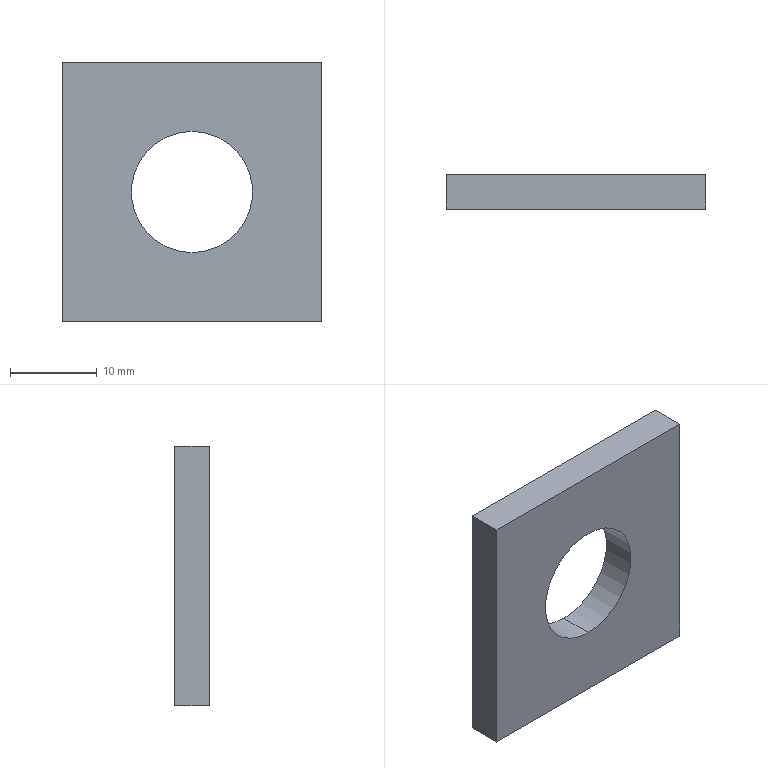Part | SolidWorks | features ICE 2, Extrusion 1 | 1 solid | 8 faces | box 30 x 4 x 30 mm | volume 2984 mm3 | plane 6 | cylinder 2 | commonest cylinder face diameters 14 x2
STEP:
#1=CARTESIAN_POINT('',(15.,0.,8.));
#2=VERTEX_POINT('',#1);
#3=CARTESIAN_POINT('',(15.,0.,22.));
#4=VERTEX_POINT('',#3);
#5=CARTESIAN_POINT('',(15.,0.,15.));
#6=DIRECTION('',(0.,1.,0.));
#7=DIRECTION('',(0.,0.,1.));
#8=AXIS2_PLACEMENT_3D('',#5,#6,#7);
#9=CIRCLE('',#8,7.);
#10=EDGE_CURVE('',#2,#4,#9,.T.);
#11=ORIENTED_EDGE('',*,*,#10,.F.);
#12=CARTESIAN_POINT('',(15.,4.,8.));
#13=VERTEX_POINT('',#12);
#14=CARTESIAN_POINT('',(15.,0.,8.));
#15=DIRECTION('',(0.,1.,0.));
#16=VECTOR('',#15,1000.);
#17=LINE('',#14,#16);
#18=EDGE_CURVE('',#2,#13,#17,.T.);
#19=ORIENTED_EDGE('',*,*,#18,.T.);
#20=CARTESIAN_POINT('',(15.,4.,22.));
#21=VERTEX_POINT('',#20);
#22=CARTESIAN_POINT('',(15.,4.,15.));
#23=DIRECTION('',(0.,1.,0.));
#24=DIRECTION('',(0.,0.,1.));
#25=AXIS2_PLACEMENT_3D('',#22,#23,#24);
#26=CIRCLE('',#25,7.);
#27=EDGE_CURVE('',#13,#21,#26,.T.);
#28=ORIENTED_EDGE('',*,*,#27,.T.);
#29=CARTESIAN_POINT('',(15.,0.,22.));
#30=DIRECTION('',(0.,1.,0.));
#31=VECTOR('',#30,1000.);
#32=LINE('',#29,#31);
#33=EDGE_CURVE('',#4,#21,#32,.T.);
#34=ORIENTED_EDGE('',*,*,#33,.F.);
#35=EDGE_LOOP('',(#11,#19,#28,#34));
#36=FACE_OUTER_BOUND('',#35,.T.);
#37=CARTESIAN_POINT('',(15.,0.,15.));
#38=DIRECTION('',(0.,1.,0.));
#39=DIRECTION('',(0.,0.,1.));
#40=AXIS2_PLACEMENT_3D('',#37,#38,#39);
#41=CYLINDRICAL_SURFACE('',#40,7.);
#42=ADVANCED_FACE('',(#36),#41,.F.);
#43=CARTESIAN_POINT('',(0.,0.,0.));
#44=VERTEX_POINT('',#43);
#45=CARTESIAN_POINT('',(0.,0.,30.));
#46=VERTEX_POINT('',#45);
#47=CARTESIAN_POINT('',(0.,0.,0.));
#48=DIRECTION('',(0.,0.,1.));
#49=VECTOR('',#48,1000.);
#50=LINE('',#47,#49);
#51=EDGE_CURVE('',#44,#46,#50,.T.);
#52=ORIENTED_EDGE('',*,*,#51,.T.);
#53=CARTESIAN_POINT('',(0.,4.,30.));
#54=VERTEX_POINT('',#53);
#55=CARTESIAN_POINT('',(0.,4.,30.));
#56=DIRECTION('',(0.,-1.,0.));
#57=VECTOR('',#56,1000.);
#58=LINE('',#55,#57);
#59=EDGE_CURVE('',#54,#46,#58,.T.);
#60=ORIENTED_EDGE('',*,*,#59,.F.);
#61=CARTESIAN_POINT('',(0.,4.,0.));
#62=VERTEX_POINT('',#61);
#63=CARTESIAN_POINT('',(0.,4.,0.));
#64=DIRECTION('',(0.,0.,1.));
#65=VECTOR('',#64,1000.);
#66=LINE('',#63,#65);
#67=EDGE_CURVE('',#62,#54,#66,.T.);
#68=ORIENTED_EDGE('',*,*,#67,.F.);
#69=CARTESIAN_POINT('',(0.,4.,0.));
#70=DIRECTION('',(0.,-1.,0.));
#71=VECTOR('',#70,1000.);
#72=LINE('',#69,#71);
#73=EDGE_CURVE('',#62,#44,#72,.T.);
#74=ORIENTED_EDGE('',*,*,#73,.T.);
#75=EDGE_LOOP('',(#52,#60,#68,#74));
#76=FACE_OUTER_BOUND('',#75,.T.);
#77=CARTESIAN_POINT('',(0.,4.,0.));
#78=DIRECTION('',(1.,0.,0.));
#79=DIRECTION('',(0.,0.,-1.));
#80=AXIS2_PLACEMENT_3D('',#77,#78,#79);
#81=PLANE('',#80);
#82=ADVANCED_FACE('',(#76),#81,.F.);
#83=CARTESIAN_POINT('',(30.,0.,30.));
#84=VERTEX_POINT('',#83);
#85=CARTESIAN_POINT('',(0.,0.,30.));
#86=DIRECTION('',(1.,0.,0.));
#87=VECTOR('',#86,1000.);
#88=LINE('',#85,#87);
#89=EDGE_CURVE('',#46,#84,#88,.T.);
#90=ORIENTED_EDGE('',*,*,#89,.T.);
#91=CARTESIAN_POINT('',(30.,4.,30.));
#92=VERTEX_POINT('',#91);
#93=CARTESIAN_POINT('',(30.,4.,30.));
#94=DIRECTION('',(0.,-1.,0.));
#95=VECTOR('',#94,1000.);
#96=LINE('',#93,#95);
#97=EDGE_CURVE('',#92,#84,#96,.T.);
#98=ORIENTED_EDGE('',*,*,#97,.F.);
#99=CARTESIAN_POINT('',(0.,4.,30.));
#100=DIRECTION('',(1.,0.,0.));
#101=VECTOR('',#100,1000.);
#102=LINE('',#99,#101);
#103=EDGE_CURVE('',#54,#92,#102,.T.);
#104=ORIENTED_EDGE('',*,*,#103,.F.);
#105=ORIENTED_EDGE('',*,*,#59,.T.);
#106=EDGE_LOOP('',(#90,#98,#104,#105));
#107=FACE_OUTER_BOUND('',#106,.T.);
#108=CARTESIAN_POINT('',(0.,4.,30.));
#109=DIRECTION('',(0.,0.,-1.));
#110=DIRECTION('',(-1.,0.,0.));
#111=AXIS2_PLACEMENT_3D('',#108,#109,#110);
#112=PLANE('',#111);
#113=ADVANCED_FACE('',(#107),#112,.F.);
#114=CARTESIAN_POINT('',(30.,0.,0.));
#115=VERTEX_POINT('',#114);
#116=CARTESIAN_POINT('',(30.,0.,0.));
#117=DIRECTION('',(0.,0.,-1.));
#118=VECTOR('',#117,1000.);
#119=LINE('',#116,#118);
#120=EDGE_CURVE('',#84,#115,#119,.T.);
#121=ORIENTED_EDGE('',*,*,#120,.T.);
#122=CARTESIAN_POINT('',(30.,4.,0.));
#123=VERTEX_POINT('',#122);
#124=CARTESIAN_POINT('',(30.,4.,0.));
#125=DIRECTION('',(0.,-1.,0.));
#126=VECTOR('',#125,1000.);
#127=LINE('',#124,#126);
#128=EDGE_CURVE('',#123,#115,#127,.T.);
#129=ORIENTED_EDGE('',*,*,#128,.F.);
#130=CARTESIAN_POINT('',(30.,4.,0.));
#131=DIRECTION('',(0.,0.,-1.));
#132=VECTOR('',#131,1000.);
#133=LINE('',#130,#132);
#134=EDGE_CURVE('',#92,#123,#133,.T.);
#135=ORIENTED_EDGE('',*,*,#134,.F.);
#136=ORIENTED_EDGE('',*,*,#97,.T.);
#137=EDGE_LOOP('',(#121,#129,#135,#136));
#138=FACE_OUTER_BOUND('',#137,.T.);
#139=CARTESIAN_POINT('',(30.,4.,0.));
#140=DIRECTION('',(-1.,0.,0.));
#141=DIRECTION('',(0.,0.,1.));
#142=AXIS2_PLACEMENT_3D('',#139,#140,#141);
#143=PLANE('',#142);
#144=ADVANCED_FACE('',(#138),#143,.F.);
#145=CARTESIAN_POINT('',(0.,0.,0.));
#146=DIRECTION('',(-1.,0.,0.));
#147=VECTOR('',#146,1000.);
#148=LINE('',#145,#147);
#149=EDGE_CURVE('',#115,#44,#148,.T.);
#150=ORIENTED_EDGE('',*,*,#149,.T.);
#151=ORIENTED_EDGE('',*,*,#73,.F.);
#152=CARTESIAN_POINT('',(0.,4.,0.));
#153=DIRECTION('',(-1.,0.,0.));
#154=VECTOR('',#153,1000.);
#155=LINE('',#152,#154);
#156=EDGE_CURVE('',#123,#62,#155,.T.);
#157=ORIENTED_EDGE('',*,*,#156,.F.);
#158=ORIENTED_EDGE('',*,*,#128,.T.);
#159=EDGE_LOOP('',(#150,#151,#157,#158));
#160=FACE_OUTER_BOUND('',#159,.T.);
#161=CARTESIAN_POINT('',(0.,4.,0.));
#162=DIRECTION('',(0.,0.,1.));
#163=DIRECTION('',(1.,0.,0.));
#164=AXIS2_PLACEMENT_3D('',#161,#162,#163);
#165=PLANE('',#164);
#166=ADVANCED_FACE('',(#160),#165,.F.);
#167=CARTESIAN_POINT('',(15.,4.,15.));
#168=DIRECTION('',(0.,1.,0.));
#169=DIRECTION('',(0.,0.,1.));
#170=AXIS2_PLACEMENT_3D('',#167,#168,#169);
#171=CIRCLE('',#170,7.);
#172=EDGE_CURVE('',#21,#13,#171,.T.);
#173=ORIENTED_EDGE('',*,*,#172,.F.);
#174=ORIENTED_EDGE('',*,*,#27,.F.);
#175=EDGE_LOOP('',(#173,#174));
#176=FACE_BOUND('',#175,.T.);
#177=ORIENTED_EDGE('',*,*,#67,.T.);
#178=ORIENTED_EDGE('',*,*,#103,.T.);
#179=ORIENTED_EDGE('',*,*,#134,.T.);
#180=ORIENTED_EDGE('',*,*,#156,.T.);
#181=EDGE_LOOP('',(#177,#178,#179,#180));
#182=FACE_OUTER_BOUND('',#181,.T.);
#183=CARTESIAN_POINT('',(0.,4.,0.));
#184=DIRECTION('',(0.,1.,0.));
#185=DIRECTION('',(0.,0.,1.));
#186=AXIS2_PLACEMENT_3D('',#183,#184,#185);
#187=PLANE('',#186);
#188=ADVANCED_FACE('',(#176,#182),#187,.T.);
#189=CARTESIAN_POINT('',(15.,0.,15.));
#190=DIRECTION('',(0.,1.,0.));
#191=DIRECTION('',(0.,0.,1.));
#192=AXIS2_PLACEMENT_3D('',#189,#190,#191);
#193=CIRCLE('',#192,7.);
#194=EDGE_CURVE('',#4,#2,#193,.T.);
#195=ORIENTED_EDGE('',*,*,#194,.T.);
#196=ORIENTED_EDGE('',*,*,#10,.T.);
#197=EDGE_LOOP('',(#195,#196));
#198=FACE_BOUND('',#197,.T.);
#199=ORIENTED_EDGE('',*,*,#51,.F.);
#200=ORIENTED_EDGE('',*,*,#149,.F.);
#201=ORIENTED_EDGE('',*,*,#120,.F.);
#202=ORIENTED_EDGE('',*,*,#89,.F.);
#203=EDGE_LOOP('',(#199,#200,#201,#202));
#204=FACE_OUTER_BOUND('',#203,.T.);
#205=CARTESIAN_POINT('',(0.,0.,0.));
#206=DIRECTION('',(0.,1.,0.));
#207=DIRECTION('',(0.,0.,1.));
#208=AXIS2_PLACEMENT_3D('',#205,#206,#207);
#209=PLANE('',#208);
#210=ADVANCED_FACE('',(#198,#204),#209,.F.);
#211=ORIENTED_EDGE('',*,*,#18,.F.);
#212=ORIENTED_EDGE('',*,*,#194,.F.);
#213=ORIENTED_EDGE('',*,*,#33,.T.);
#214=ORIENTED_EDGE('',*,*,#172,.T.);
#215=EDGE_LOOP('',(#211,#212,#213,#214));
#216=FACE_OUTER_BOUND('',#215,.T.);
#217=CARTESIAN_POINT('',(15.,0.,15.));
#218=DIRECTION('',(0.,1.,0.));
#219=DIRECTION('',(0.,0.,1.));
#220=AXIS2_PLACEMENT_3D('',#217,#218,#219);
#221=CYLINDRICAL_SURFACE('',#220,7.);
#222=ADVANCED_FACE('',(#216),#221,.F.);
#223=CLOSED_SHELL('',(#42,#82,#113,#144,#166,#188,#210,#222));
#224=MANIFOLD_SOLID_BREP('',#223);
#225=CARTESIAN_POINT('',(0.,0.,0.));
#226=DIRECTION('',(0.,0.,1.));
#227=DIRECTION('',(1.,0.,0.));
#228=AXIS2_PLACEMENT_3D('',#225,#226,#227);
#229=(LENGTH_UNIT()NAMED_UNIT(*)SI_UNIT(.MILLI.,.METRE.));
#230=UNCERTAINTY_MEASURE_WITH_UNIT(LENGTH_MEASURE(0.00001),#229,'','');
#231=(NAMED_UNIT(*)PLANE_ANGLE_UNIT()SI_UNIT($,.RADIAN.));
#232=(NAMED_UNIT(*)SI_UNIT($,.STERADIAN.)SOLID_ANGLE_UNIT());
#233=(GEOMETRIC_REPRESENTATION_CONTEXT(3)GLOBAL_UNCERTAINTY_ASSIGNED_CONTEXT((#230))GLOBAL_UNIT_ASSIGNED_CONTEXT((#229,#231,#232))REPRESENTATION_CONTEXT('',''));
#234=ADVANCED_BREP_SHAPE_REPRESENTATION('',(#224,#228),#233);